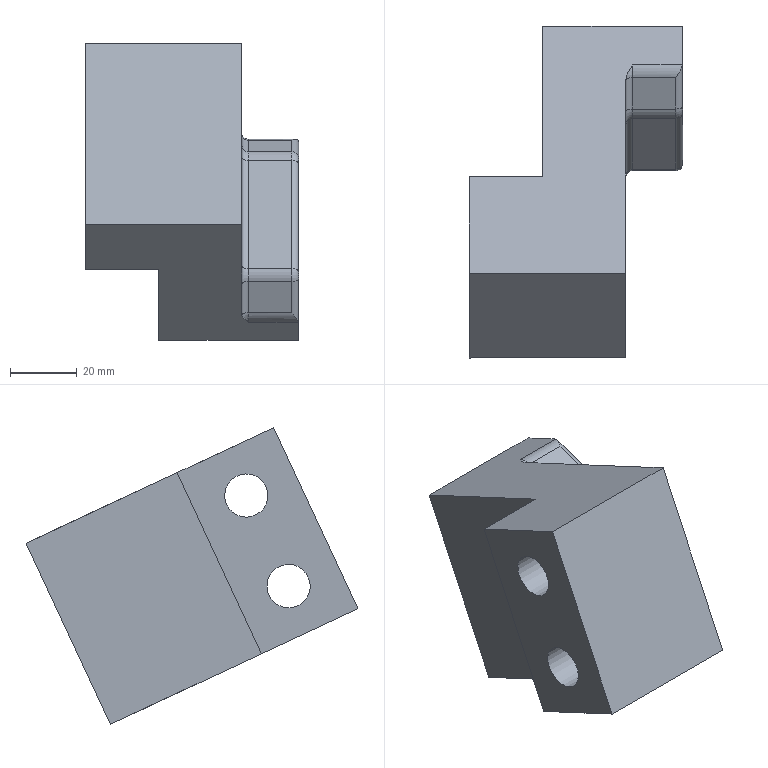Part | NX | features MAIN_BODY 2 | 1 solid | 34 faces | box 64 x 99.674 x 89.033 mm | volume 166732 mm3 | plane 14 | cylinder 14 | torus 6 | commonest cylinder face diameters 4 x6 10 x4 13 x2 20 x2
STEP:
#1=CARTESIAN_POINT('',(570.,631.034,-80.229));
#2=VERTEX_POINT('',#1);
#3=CARTESIAN_POINT('',(570.,656.391,-25.851));
#4=VERTEX_POINT('',#3);
#5=CARTESIAN_POINT('',(570.,631.034,-80.229));
#6=DIRECTION('',(0.,0.4226,0.9063));
#7=VECTOR('',#6,1000.);
#8=LINE('',#5,#7);
#9=EDGE_CURVE('',#2,#4,#8,.T.);
#10=ORIENTED_EDGE('',*,*,#9,.T.);
#11=CARTESIAN_POINT('',(570.,701.706,-46.982));
#12=VERTEX_POINT('',#11);
#13=CARTESIAN_POINT('',(570.,701.706,-46.982));
#14=DIRECTION('',(0.,-0.9063,0.4226));
#15=VECTOR('',#14,1000.);
#16=LINE('',#13,#15);
#17=EDGE_CURVE('',#12,#4,#16,.T.);
#18=ORIENTED_EDGE('',*,*,#17,.F.);
#19=CARTESIAN_POINT('',(570.,676.349,-101.36));
#20=VERTEX_POINT('',#19);
#21=CARTESIAN_POINT('',(570.,657.331,-142.144));
#22=DIRECTION('',(0.,0.4226,0.9063));
#23=VECTOR('',#22,1000.);
#24=LINE('',#21,#23);
#25=EDGE_CURVE('',#20,#12,#24,.T.);
#26=ORIENTED_EDGE('',*,*,#25,.F.);
#27=CARTESIAN_POINT('',(570.,676.349,-101.36));
#28=DIRECTION('',(0.,0.9063,-0.4226));
#29=VECTOR('',#28,1000.);
#30=LINE('',#27,#29);
#31=EDGE_CURVE('',#20,#2,#30,.F.);
#32=ORIENTED_EDGE('',*,*,#31,.T.);
#33=EDGE_LOOP('',(#10,#18,#26,#32));
#34=FACE_BOUND('',#33,.T.);
#35=CARTESIAN_POINT('',(570.,657.331,-142.144));
#36=DIRECTION('',(1.,0.,0.));
#37=DIRECTION('',(0.,-0.8192,-0.5736));
#38=AXIS2_PLACEMENT_3D('',#35,#36,#37);
#39=PLANE('',#38);
#40=ADVANCED_FACE('',(#34),#39,.F.);
#41=CARTESIAN_POINT('',(597.,689.989,-41.518));
#42=VERTEX_POINT('',#41);
#43=CARTESIAN_POINT('',(611.927,689.989,-41.518));
#44=VERTEX_POINT('',#43);
#45=CARTESIAN_POINT('',(563.,689.989,-41.518));
#46=DIRECTION('',(1.,0.,0.));
#47=VECTOR('',#46,1000.);
#48=LINE('',#45,#47);
#49=EDGE_CURVE('',#42,#44,#48,.T.);
#50=ORIENTED_EDGE('',*,*,#49,.T.);
#51=CARTESIAN_POINT('',(612.,690.675,-41.838));
#52=VERTEX_POINT('',#51);
#53=CARTESIAN_POINT('',(610.,690.675,-41.838));
#54=DIRECTION('',(0.,0.4226,0.9063));
#55=DIRECTION('',(0.,-0.9063,0.4226));
#56=AXIS2_PLACEMENT_3D('',#53,#54,#55);
#57=ELLIPSE('',#56,2.828,2.);
#58=EDGE_CURVE('',#44,#52,#57,.T.);
#59=ORIENTED_EDGE('',*,*,#58,.T.);
#60=CARTESIAN_POINT('',(612.,701.706,-46.982));
#61=VERTEX_POINT('',#60);
#62=CARTESIAN_POINT('',(612.,701.706,-46.982));
#63=DIRECTION('',(0.,-0.9063,0.4226));
#64=VECTOR('',#63,1000.);
#65=LINE('',#62,#64);
#66=EDGE_CURVE('',#61,#52,#65,.T.);
#67=ORIENTED_EDGE('',*,*,#66,.F.);
#68=CARTESIAN_POINT('',(563.,701.706,-46.982));
#69=DIRECTION('',(1.,0.,0.));
#70=VECTOR('',#69,1000.);
#71=LINE('',#68,#70);
#72=EDGE_CURVE('',#12,#61,#71,.T.);
#73=ORIENTED_EDGE('',*,*,#72,.F.);
#74=ORIENTED_EDGE('',*,*,#17,.T.);
#75=CARTESIAN_POINT('',(548.,656.391,-25.851));
#76=VERTEX_POINT('',#75);
#77=CARTESIAN_POINT('',(570.,656.391,-25.851));
#78=DIRECTION('',(1.,0.,0.));
#79=VECTOR('',#78,1000.);
#80=LINE('',#77,#79);
#81=EDGE_CURVE('',#4,#76,#80,.F.);
#82=ORIENTED_EDGE('',*,*,#81,.T.);
#83=CARTESIAN_POINT('',(548.,627.389,-12.327));
#84=VERTEX_POINT('',#83);
#85=CARTESIAN_POINT('',(548.,627.389,-12.327));
#86=DIRECTION('',(0.,0.9063,-0.4226));
#87=VECTOR('',#86,1000.);
#88=LINE('',#85,#87);
#89=EDGE_CURVE('',#84,#76,#88,.T.);
#90=ORIENTED_EDGE('',*,*,#89,.F.);
#91=CARTESIAN_POINT('',(595.,627.389,-12.327));
#92=VERTEX_POINT('',#91);
#93=CARTESIAN_POINT('',(563.,627.389,-12.327));
#94=DIRECTION('',(-1.,0.,0.));
#95=VECTOR('',#94,1000.);
#96=LINE('',#93,#95);
#97=EDGE_CURVE('',#84,#92,#96,.F.);
#98=ORIENTED_EDGE('',*,*,#97,.T.);
#99=CARTESIAN_POINT('',(595.,685.549,-39.447));
#100=VERTEX_POINT('',#99);
#101=CARTESIAN_POINT('',(595.,679.049,-36.416));
#102=DIRECTION('',(0.,-0.9063,0.4226));
#103=VECTOR('',#102,1000.);
#104=LINE('',#101,#103);
#105=EDGE_CURVE('',#100,#92,#104,.T.);
#106=ORIENTED_EDGE('',*,*,#105,.F.);
#107=CARTESIAN_POINT('',(595.,685.549,-39.447));
#108=CARTESIAN_POINT('',(595.,686.371,-39.831));
#109=CARTESIAN_POINT('',(595.571,687.945,-40.564));
#110=CARTESIAN_POINT('',(596.522,689.304,-41.198));
#111=CARTESIAN_POINT('',(597.,689.989,-41.518));
#112=B_SPLINE_CURVE_WITH_KNOTS('',3,(#107,#108,#109,#110,#111),.UNSPECIFIED.,.F.,.F.,(4,1,4),(0.,0.002683,0.005365),.UNSPECIFIED.);
#113=EDGE_CURVE('',#100,#42,#112,.T.);
#114=ORIENTED_EDGE('',*,*,#113,.T.);
#115=EDGE_LOOP('',(#50,#59,#67,#73,#74,#82,#90,#98,#106,#114));
#116=FACE_BOUND('',#115,.T.);
#117=CARTESIAN_POINT('',(563.,701.706,-46.982));
#118=DIRECTION('',(0.,0.4226,0.9063));
#119=DIRECTION('',(0.,-0.9063,0.4226));
#120=AXIS2_PLACEMENT_3D('',#117,#118,#119);
#121=PLANE('',#120);
#122=ADVANCED_FACE('',(#116),#121,.T.);
#123=CARTESIAN_POINT('',(548.,602.032,-66.705));
#124=VERTEX_POINT('',#123);
#125=CARTESIAN_POINT('',(595.,602.032,-66.705));
#126=VERTEX_POINT('',#125);
#127=CARTESIAN_POINT('',(563.,602.032,-66.705));
#128=DIRECTION('',(1.,0.,0.));
#129=VECTOR('',#128,1000.);
#130=LINE('',#127,#129);
#131=EDGE_CURVE('',#124,#126,#130,.T.);
#132=ORIENTED_EDGE('',*,*,#131,.T.);
#133=CARTESIAN_POINT('',(595.,583.014,-107.489));
#134=DIRECTION('',(0.,-0.4226,-0.9063));
#135=VECTOR('',#134,1000.);
#136=LINE('',#133,#135);
#137=EDGE_CURVE('',#126,#92,#136,.F.);
#138=ORIENTED_EDGE('',*,*,#137,.T.);
#139=ORIENTED_EDGE('',*,*,#97,.F.);
#140=CARTESIAN_POINT('',(548.,602.032,-66.705));
#141=DIRECTION('',(0.,0.4226,0.9063));
#142=VECTOR('',#141,1000.);
#143=LINE('',#140,#142);
#144=EDGE_CURVE('',#124,#84,#143,.T.);
#145=ORIENTED_EDGE('',*,*,#144,.F.);
#146=EDGE_LOOP('',(#132,#138,#139,#145));
#147=FACE_BOUND('',#146,.T.);
#148=CARTESIAN_POINT('',(563.,583.014,-107.489));
#149=DIRECTION('',(0.,0.9063,-0.4226));
#150=DIRECTION('',(0.,0.4226,0.9063));
#151=AXIS2_PLACEMENT_3D('',#148,#149,#150);
#152=PLANE('',#151);
#153=ADVANCED_FACE('',(#147),#152,.F.);
#154=CARTESIAN_POINT('',(612.,676.349,-101.36));
#155=VERTEX_POINT('',#154);
#156=CARTESIAN_POINT('',(612.,665.318,-96.216));
#157=VERTEX_POINT('',#156);
#158=CARTESIAN_POINT('',(612.,676.349,-101.36));
#159=DIRECTION('',(0.,0.9063,-0.4226));
#160=VECTOR('',#159,1000.);
#161=LINE('',#158,#160);
#162=EDGE_CURVE('',#155,#157,#161,.F.);
#163=ORIENTED_EDGE('',*,*,#162,.T.);
#164=CARTESIAN_POINT('',(611.927,664.632,-95.896));
#165=VERTEX_POINT('',#164);
#166=CARTESIAN_POINT('',(610.,665.318,-96.216));
#167=DIRECTION('',(0.,0.4226,0.9063));
#168=DIRECTION('',(0.,-0.9063,0.4226));
#169=AXIS2_PLACEMENT_3D('',#166,#167,#168);
#170=ELLIPSE('',#169,2.828,2.);
#171=EDGE_CURVE('',#157,#165,#170,.F.);
#172=ORIENTED_EDGE('',*,*,#171,.T.);
#173=CARTESIAN_POINT('',(597.,664.632,-95.896));
#174=VERTEX_POINT('',#173);
#175=CARTESIAN_POINT('',(563.,664.632,-95.896));
#176=DIRECTION('',(1.,0.,0.));
#177=VECTOR('',#176,1000.);
#178=LINE('',#175,#177);
#179=EDGE_CURVE('',#165,#174,#178,.F.);
#180=ORIENTED_EDGE('',*,*,#179,.T.);
#181=CARTESIAN_POINT('',(595.,660.192,-93.826));
#182=VERTEX_POINT('',#181);
#183=CARTESIAN_POINT('',(595.,660.192,-93.826));
#184=CARTESIAN_POINT('',(595.,661.014,-94.209));
#185=CARTESIAN_POINT('',(595.571,662.587,-94.943));
#186=CARTESIAN_POINT('',(596.522,663.947,-95.577));
#187=CARTESIAN_POINT('',(597.,664.632,-95.896));
#188=B_SPLINE_CURVE_WITH_KNOTS('',3,(#183,#184,#185,#186,#187),.UNSPECIFIED.,.F.,.F.,(4,1,4),(0.,0.002683,0.005365),.UNSPECIFIED.);
#189=EDGE_CURVE('',#174,#182,#188,.F.);
#190=ORIENTED_EDGE('',*,*,#189,.T.);
#191=CARTESIAN_POINT('',(595.,653.692,-90.795));
#192=DIRECTION('',(0.,-0.9063,0.4226));
#193=VECTOR('',#192,1000.);
#194=LINE('',#191,#193);
#195=EDGE_CURVE('',#182,#126,#194,.T.);
#196=ORIENTED_EDGE('',*,*,#195,.T.);
#197=ORIENTED_EDGE('',*,*,#131,.F.);
#198=CARTESIAN_POINT('',(548.,631.034,-80.229));
#199=VERTEX_POINT('',#198);
#200=CARTESIAN_POINT('',(548.,602.032,-66.705));
#201=DIRECTION('',(0.,0.9063,-0.4226));
#202=VECTOR('',#201,1000.);
#203=LINE('',#200,#202);
#204=EDGE_CURVE('',#124,#199,#203,.T.);
#205=ORIENTED_EDGE('',*,*,#204,.T.);
#206=CARTESIAN_POINT('',(570.,631.034,-80.229));
#207=DIRECTION('',(1.,0.,0.));
#208=VECTOR('',#207,1000.);
#209=LINE('',#206,#208);
#210=EDGE_CURVE('',#2,#199,#209,.F.);
#211=ORIENTED_EDGE('',*,*,#210,.F.);
#212=ORIENTED_EDGE('',*,*,#31,.F.);
#213=CARTESIAN_POINT('',(563.,676.349,-101.36));
#214=DIRECTION('',(-1.,0.,0.));
#215=VECTOR('',#214,1000.);
#216=LINE('',#213,#215);
#217=EDGE_CURVE('',#20,#155,#216,.F.);
#218=ORIENTED_EDGE('',*,*,#217,.T.);
#219=EDGE_LOOP('',(#163,#172,#180,#190,#196,#197,#205,#211,#212,#218));
#220=FACE_BOUND('',#219,.T.);
#221=CARTESIAN_POINT('',(563.,676.349,-101.36));
#222=DIRECTION('',(0.,0.4226,0.9063));
#223=DIRECTION('',(0.,-0.9063,0.4226));
#224=AXIS2_PLACEMENT_3D('',#221,#222,#223);
#225=PLANE('',#224);
#226=ADVANCED_FACE('',(#220),#225,.F.);
#227=CARTESIAN_POINT('',(612.,660.606,-80.7));
#228=VERTEX_POINT('',#227);
#229=CARTESIAN_POINT('',(612.,660.506,-82.994));
#230=VERTEX_POINT('',#229);
#231=CARTESIAN_POINT('',(612.,663.325,-81.968));
#232=DIRECTION('',(1.,0.,0.));
#233=DIRECTION('',(0.,-0.8192,-0.5736));
#234=AXIS2_PLACEMENT_3D('',#231,#232,#233);
#235=CIRCLE('',#234,3.);
#236=EDGE_CURVE('',#228,#230,#235,.T.);
#237=ORIENTED_EDGE('',*,*,#236,.T.);
#238=CARTESIAN_POINT('',(612.,679.145,-134.205));
#239=DIRECTION('',(0.,-0.342,0.9397));
#240=VECTOR('',#239,1000.);
#241=LINE('',#238,#240);
#242=EDGE_CURVE('',#230,#157,#241,.F.);
#243=ORIENTED_EDGE('',*,*,#242,.T.);
#244=ORIENTED_EDGE('',*,*,#162,.F.);
#245=CARTESIAN_POINT('',(612.,657.331,-142.144));
#246=DIRECTION('',(0.,0.4226,0.9063));
#247=VECTOR('',#246,1000.);
#248=LINE('',#245,#247);
#249=EDGE_CURVE('',#155,#61,#248,.T.);
#250=ORIENTED_EDGE('',*,*,#249,.T.);
#251=ORIENTED_EDGE('',*,*,#66,.T.);
#252=CARTESIAN_POINT('',(612.,677.453,-46.65));
#253=VERTEX_POINT('',#252);
#254=CARTESIAN_POINT('',(612.,628.994,-64.288));
#255=DIRECTION('',(0.,-0.9397,-0.342));
#256=VECTOR('',#255,1000.);
#257=LINE('',#254,#256);
#258=EDGE_CURVE('',#52,#253,#257,.T.);
#259=ORIENTED_EDGE('',*,*,#258,.T.);
#260=CARTESIAN_POINT('',(612.,675.76,-48.202));
#261=VERTEX_POINT('',#260);
#262=CARTESIAN_POINT('',(612.,678.479,-49.469));
#263=DIRECTION('',(1.,0.,0.));
#264=DIRECTION('',(0.,-0.8192,-0.5736));
#265=AXIS2_PLACEMENT_3D('',#262,#263,#264);
#266=CIRCLE('',#265,3.);
#267=EDGE_CURVE('',#253,#261,#266,.T.);
#268=ORIENTED_EDGE('',*,*,#267,.T.);
#269=CARTESIAN_POINT('',(612.,636.486,-132.424));
#270=DIRECTION('',(0.,0.4226,0.9063));
#271=VECTOR('',#270,1000.);
#272=LINE('',#269,#271);
#273=EDGE_CURVE('',#261,#228,#272,.F.);
#274=ORIENTED_EDGE('',*,*,#273,.T.);
#275=EDGE_LOOP('',(#237,#243,#244,#250,#251,#259,#268,#274));
#276=FACE_BOUND('',#275,.T.);
#277=CARTESIAN_POINT('',(612.,657.331,-142.144));
#278=DIRECTION('',(1.,0.,0.));
#279=DIRECTION('',(0.,-0.8192,-0.5736));
#280=AXIS2_PLACEMENT_3D('',#277,#278,#279);
#281=PLANE('',#280);
#282=ADVANCED_FACE('',(#276),#281,.T.);
#283=ORIENTED_EDGE('',*,*,#217,.F.);
#284=ORIENTED_EDGE('',*,*,#25,.T.);
#285=ORIENTED_EDGE('',*,*,#72,.T.);
#286=ORIENTED_EDGE('',*,*,#249,.F.);
#287=EDGE_LOOP('',(#283,#284,#285,#286));
#288=FACE_BOUND('',#287,.T.);
#289=CARTESIAN_POINT('',(563.,657.331,-142.144));
#290=DIRECTION('',(0.,0.9063,-0.4226));
#291=DIRECTION('',(0.,0.4226,0.9063));
#292=AXIS2_PLACEMENT_3D('',#289,#290,#291);
#293=PLANE('',#292);
#294=ADVANCED_FACE('',(#288),#293,.T.);
#295=CARTESIAN_POINT('',(597.,658.793,-79.855));
#296=VERTEX_POINT('',#295);
#297=CARTESIAN_POINT('',(610.,658.793,-79.855));
#298=VERTEX_POINT('',#297);
#299=CARTESIAN_POINT('',(563.,658.793,-79.855));
#300=DIRECTION('',(-1.,0.,0.));
#301=VECTOR('',#300,1000.);
#302=LINE('',#299,#301);
#303=EDGE_CURVE('',#296,#298,#302,.F.);
#304=ORIENTED_EDGE('',*,*,#303,.T.);
#305=CARTESIAN_POINT('',(610.,673.947,-47.356));
#306=VERTEX_POINT('',#305);
#307=CARTESIAN_POINT('',(610.,653.692,-90.795));
#308=DIRECTION('',(0.,-0.4226,-0.9063));
#309=VECTOR('',#308,1000.);
#310=LINE('',#307,#309);
#311=EDGE_CURVE('',#298,#306,#310,.F.);
#312=ORIENTED_EDGE('',*,*,#311,.T.);
#313=CARTESIAN_POINT('',(597.,673.947,-47.356));
#314=VERTEX_POINT('',#313);
#315=CARTESIAN_POINT('',(563.,673.947,-47.356));
#316=DIRECTION('',(-1.,0.,0.));
#317=VECTOR('',#316,1000.);
#318=LINE('',#315,#317);
#319=EDGE_CURVE('',#306,#314,#318,.T.);
#320=ORIENTED_EDGE('',*,*,#319,.T.);
#321=CARTESIAN_POINT('',(597.,658.793,-79.855));
#322=DIRECTION('',(0.,0.4226,0.9063));
#323=VECTOR('',#322,1000.);
#324=LINE('',#321,#323);
#325=EDGE_CURVE('',#314,#296,#324,.F.);
#326=ORIENTED_EDGE('',*,*,#325,.T.);
#327=EDGE_LOOP('',(#304,#312,#320,#326));
#328=FACE_BOUND('',#327,.T.);
#329=CARTESIAN_POINT('',(563.,653.692,-90.795));
#330=DIRECTION('',(0.,0.9063,-0.4226));
#331=DIRECTION('',(0.,0.4226,0.9063));
#332=AXIS2_PLACEMENT_3D('',#329,#330,#331);
#333=PLANE('',#332);
#334=ADVANCED_FACE('',(#328),#333,.F.);
#335=CARTESIAN_POINT('',(595.,625.46,-50.213));
#336=VERTEX_POINT('',#335);
#337=CARTESIAN_POINT('',(595.,622.872,-59.873));
#338=DIRECTION('',(-1.,0.,0.));
#339=DIRECTION('',(0.,0.2588,0.9659));
#340=AXIS2_PLACEMENT_3D('',#337,#338,#339);
#341=CIRCLE('',#340,10.);
#342=EDGE_CURVE('',#336,#336,#341,.T.);
#343=ORIENTED_EDGE('',*,*,#342,.T.);
#344=EDGE_LOOP('',(#343));
#345=FACE_BOUND('',#344,.T.);
#346=CARTESIAN_POINT('',(595.,638.139,-23.024));
#347=VERTEX_POINT('',#346);
#348=CARTESIAN_POINT('',(595.,635.551,-32.683));
#349=DIRECTION('',(-1.,0.,0.));
#350=DIRECTION('',(0.,0.2588,0.9659));
#351=AXIS2_PLACEMENT_3D('',#348,#349,#350);
#352=CIRCLE('',#351,10.);
#353=EDGE_CURVE('',#347,#347,#352,.T.);
#354=ORIENTED_EDGE('',*,*,#353,.T.);
#355=EDGE_LOOP('',(#354));
#356=FACE_BOUND('',#355,.T.);
#357=ORIENTED_EDGE('',*,*,#195,.F.);
#358=CARTESIAN_POINT('',(595.,660.167,-93.759));
#359=VERTEX_POINT('',#358);
#360=CARTESIAN_POINT('',(595.,666.745,-91.365));
#361=DIRECTION('',(1.,0.,0.));
#362=DIRECTION('',(0.,-0.8192,-0.5736));
#363=AXIS2_PLACEMENT_3D('',#360,#361,#362);
#364=CIRCLE('',#363,7.);
#365=EDGE_CURVE('',#182,#359,#364,.F.);
#366=ORIENTED_EDGE('',*,*,#365,.T.);
#367=CARTESIAN_POINT('',(595.,656.747,-84.362));
#368=VERTEX_POINT('',#367);
#369=CARTESIAN_POINT('',(595.,656.747,-84.362));
#370=DIRECTION('',(0.,0.342,-0.9397));
#371=VECTOR('',#370,1000.);
#372=LINE('',#369,#371);
#373=EDGE_CURVE('',#359,#368,#372,.F.);
#374=ORIENTED_EDGE('',*,*,#373,.T.);
#375=CARTESIAN_POINT('',(595.,656.98,-79.009));
#376=VERTEX_POINT('',#375);
#377=CARTESIAN_POINT('',(595.,663.325,-81.968));
#378=DIRECTION('',(1.,0.,0.));
#379=DIRECTION('',(0.,-0.8192,-0.5736));
#380=AXIS2_PLACEMENT_3D('',#377,#378,#379);
#381=CIRCLE('',#380,7.);
#382=EDGE_CURVE('',#368,#376,#381,.F.);
#383=ORIENTED_EDGE('',*,*,#382,.T.);
#384=CARTESIAN_POINT('',(595.,672.135,-46.511));
#385=VERTEX_POINT('',#384);
#386=CARTESIAN_POINT('',(595.,672.135,-46.511));
#387=DIRECTION('',(0.,-0.4226,-0.9063));
#388=VECTOR('',#387,1000.);
#389=LINE('',#386,#388);
#390=EDGE_CURVE('',#376,#385,#389,.F.);
#391=ORIENTED_EDGE('',*,*,#390,.T.);
#392=CARTESIAN_POINT('',(595.,676.085,-42.892));
#393=VERTEX_POINT('',#392);
#394=CARTESIAN_POINT('',(595.,678.479,-49.469));
#395=DIRECTION('',(1.,0.,0.));
#396=DIRECTION('',(0.,-0.8192,-0.5736));
#397=AXIS2_PLACEMENT_3D('',#394,#395,#396);
#398=CIRCLE('',#397,7.);
#399=EDGE_CURVE('',#385,#393,#398,.F.);
#400=ORIENTED_EDGE('',*,*,#399,.T.);
#401=CARTESIAN_POINT('',(595.,685.482,-39.471));
#402=VERTEX_POINT('',#401);
#403=CARTESIAN_POINT('',(595.,685.482,-39.471));
#404=DIRECTION('',(0.,0.9397,0.342));
#405=VECTOR('',#404,1000.);
#406=LINE('',#403,#405);
#407=EDGE_CURVE('',#393,#402,#406,.T.);
#408=ORIENTED_EDGE('',*,*,#407,.T.);
#409=CARTESIAN_POINT('',(595.,687.876,-46.049));
#410=DIRECTION('',(1.,0.,0.));
#411=DIRECTION('',(0.,-0.8192,-0.5736));
#412=AXIS2_PLACEMENT_3D('',#409,#410,#411);
#413=CIRCLE('',#412,7.);
#414=EDGE_CURVE('',#402,#100,#413,.F.);
#415=ORIENTED_EDGE('',*,*,#414,.T.);
#416=ORIENTED_EDGE('',*,*,#105,.T.);
#417=ORIENTED_EDGE('',*,*,#137,.F.);
#418=EDGE_LOOP('',(#357,#366,#374,#383,#391,#400,#408,#415,#416,#417));
#419=FACE_BOUND('',#418,.T.);
#420=CARTESIAN_POINT('',(595.,653.692,-90.795));
#421=DIRECTION('',(1.,0.,0.));
#422=DIRECTION('',(0.,-0.8192,-0.5736));
#423=AXIS2_PLACEMENT_3D('',#420,#421,#422);
#424=PLANE('',#423);
#425=ADVANCED_FACE('',(#345,#356,#419),#424,.T.);
#426=CARTESIAN_POINT('',(597.,662.046,-93.075));
#427=VERTEX_POINT('',#426);
#428=CARTESIAN_POINT('',(610.,662.046,-93.075));
#429=VERTEX_POINT('',#428);
#430=CARTESIAN_POINT('',(563.,662.046,-93.075));
#431=DIRECTION('',(1.,0.,0.));
#432=VECTOR('',#431,1000.);
#433=LINE('',#430,#432);
#434=EDGE_CURVE('',#427,#429,#433,.T.);
#435=ORIENTED_EDGE('',*,*,#434,.T.);
#436=CARTESIAN_POINT('',(610.,658.626,-83.678));
#437=VERTEX_POINT('',#436);
#438=CARTESIAN_POINT('',(610.,662.755,-95.021));
#439=DIRECTION('',(0.,0.342,-0.9397));
#440=VECTOR('',#439,1000.);
#441=LINE('',#438,#440);
#442=EDGE_CURVE('',#429,#437,#441,.F.);
#443=ORIENTED_EDGE('',*,*,#442,.T.);
#444=CARTESIAN_POINT('',(597.,658.626,-83.678));
#445=VERTEX_POINT('',#444);
#446=CARTESIAN_POINT('',(563.,658.626,-83.678));
#447=DIRECTION('',(-1.,0.,0.));
#448=VECTOR('',#447,1000.);
#449=LINE('',#446,#448);
#450=EDGE_CURVE('',#437,#445,#449,.T.);
#451=ORIENTED_EDGE('',*,*,#450,.T.);
#452=CARTESIAN_POINT('',(597.,662.046,-93.075));
#453=DIRECTION('',(0.,-0.342,0.9397));
#454=VECTOR('',#453,1000.);
#455=LINE('',#452,#454);
#456=EDGE_CURVE('',#445,#427,#455,.F.);
#457=ORIENTED_EDGE('',*,*,#456,.T.);
#458=EDGE_LOOP('',(#435,#443,#451,#457));
#459=FACE_BOUND('',#458,.T.);
#460=CARTESIAN_POINT('',(563.,662.755,-95.021));
#461=DIRECTION('',(0.,0.9397,0.342));
#462=DIRECTION('',(0.,-0.342,0.9397));
#463=AXIS2_PLACEMENT_3D('',#460,#461,#462);
#464=PLANE('',#463);
#465=ADVANCED_FACE('',(#459),#464,.F.);
#466=CARTESIAN_POINT('',(597.,676.769,-44.771));
#467=VERTEX_POINT('',#466);
#468=CARTESIAN_POINT('',(610.,676.769,-44.771));
#469=VERTEX_POINT('',#468);
#470=CARTESIAN_POINT('',(563.,676.769,-44.771));
#471=DIRECTION('',(1.,0.,0.));
#472=VECTOR('',#471,1000.);
#473=LINE('',#470,#472);
#474=EDGE_CURVE('',#467,#469,#473,.T.);
#475=ORIENTED_EDGE('',*,*,#474,.T.);
#476=CARTESIAN_POINT('',(610.,686.166,-41.351));
#477=VERTEX_POINT('',#476);
#478=CARTESIAN_POINT('',(610.,674.823,-45.479));
#479=DIRECTION('',(0.,-0.9397,-0.342));
#480=VECTOR('',#479,1000.);
#481=LINE('',#478,#480);
#482=EDGE_CURVE('',#469,#477,#481,.F.);
#483=ORIENTED_EDGE('',*,*,#482,.T.);
#484=CARTESIAN_POINT('',(597.,686.166,-41.351));
#485=VERTEX_POINT('',#484);
#486=CARTESIAN_POINT('',(563.,686.166,-41.351));
#487=DIRECTION('',(1.,0.,0.));
#488=VECTOR('',#487,1000.);
#489=LINE('',#486,#488);
#490=EDGE_CURVE('',#477,#485,#489,.F.);
#491=ORIENTED_EDGE('',*,*,#490,.T.);
#492=CARTESIAN_POINT('',(597.,676.769,-44.771));
#493=DIRECTION('',(0.,0.9397,0.342));
#494=VECTOR('',#493,1000.);
#495=LINE('',#492,#494);
#496=EDGE_CURVE('',#485,#467,#495,.F.);
#497=ORIENTED_EDGE('',*,*,#496,.T.);
#498=EDGE_LOOP('',(#475,#483,#491,#497));
#499=FACE_BOUND('',#498,.T.);
#500=CARTESIAN_POINT('',(563.,674.823,-45.479));
#501=DIRECTION('',(0.,-0.342,0.9397));
#502=DIRECTION('',(0.,-0.9397,-0.342));
#503=AXIS2_PLACEMENT_3D('',#500,#501,#502);
#504=PLANE('',#503);
#505=ADVANCED_FACE('',(#499),#504,.T.);
#506=ORIENTED_EDGE('',*,*,#490,.F.);
#507=CARTESIAN_POINT('',(611.927,689.989,-41.518));
#508=CARTESIAN_POINT('',(611.641,688.67,-40.903));
#509=CARTESIAN_POINT('',(610.781,687.326,-40.928));
#510=CARTESIAN_POINT('',(610.,686.166,-41.351));
#511=B_SPLINE_CURVE_WITH_KNOTS('',3,(#507,#508,#509,#510),.UNSPECIFIED.,.F.,.F.,(4,4),(0.,0.004383),.UNSPECIFIED.);
#512=EDGE_CURVE('',#477,#44,#511,.F.);
#513=ORIENTED_EDGE('',*,*,#512,.T.);
#514=ORIENTED_EDGE('',*,*,#49,.F.);
#515=CARTESIAN_POINT('',(597.,687.876,-46.049));
#516=DIRECTION('',(1.,0.,0.));
#517=DIRECTION('',(0.,-0.8192,-0.5736));
#518=AXIS2_PLACEMENT_3D('',#515,#516,#517);
#519=CIRCLE('',#518,5.);
#520=EDGE_CURVE('',#42,#485,#519,.T.);
#521=ORIENTED_EDGE('',*,*,#520,.T.);
#522=EDGE_LOOP('',(#506,#513,#514,#521));
#523=FACE_BOUND('',#522,.T.);
#524=CARTESIAN_POINT('',(563.,687.876,-46.049));
#525=DIRECTION('',(1.,0.,0.));
#526=DIRECTION('',(0.,-0.8192,-0.5736));
#527=AXIS2_PLACEMENT_3D('',#524,#525,#526);
#528=CYLINDRICAL_SURFACE('',#527,5.);
#529=ADVANCED_FACE('',(#523),#528,.T.);
#530=ORIENTED_EDGE('',*,*,#319,.F.);
#531=CARTESIAN_POINT('',(610.,678.479,-49.469));
#532=DIRECTION('',(1.,0.,0.));
#533=DIRECTION('',(0.,-0.8192,-0.5736));
#534=AXIS2_PLACEMENT_3D('',#531,#532,#533);
#535=CIRCLE('',#534,5.);
#536=EDGE_CURVE('',#306,#469,#535,.F.);
#537=ORIENTED_EDGE('',*,*,#536,.T.);
#538=ORIENTED_EDGE('',*,*,#474,.F.);
#539=CARTESIAN_POINT('',(597.,678.479,-49.469));
#540=DIRECTION('',(1.,0.,0.));
#541=DIRECTION('',(0.,-0.8192,-0.5736));
#542=AXIS2_PLACEMENT_3D('',#539,#540,#541);
#543=CIRCLE('',#542,5.);
#544=EDGE_CURVE('',#467,#314,#543,.T.);
#545=ORIENTED_EDGE('',*,*,#544,.T.);
#546=EDGE_LOOP('',(#530,#537,#538,#545));
#547=FACE_BOUND('',#546,.T.);
#548=CARTESIAN_POINT('',(563.,678.479,-49.469));
#549=DIRECTION('',(1.,0.,0.));
#550=DIRECTION('',(0.,-0.8192,-0.5736));
#551=AXIS2_PLACEMENT_3D('',#548,#549,#550);
#552=CYLINDRICAL_SURFACE('',#551,5.);
#553=ADVANCED_FACE('',(#547),#552,.T.);
#554=ORIENTED_EDGE('',*,*,#450,.F.);
#555=CARTESIAN_POINT('',(610.,663.325,-81.968));
#556=DIRECTION('',(1.,0.,0.));
#557=DIRECTION('',(0.,-0.8192,-0.5736));
#558=AXIS2_PLACEMENT_3D('',#555,#556,#557);
#559=CIRCLE('',#558,5.);
#560=EDGE_CURVE('',#437,#298,#559,.F.);
#561=ORIENTED_EDGE('',*,*,#560,.T.);
#562=ORIENTED_EDGE('',*,*,#303,.F.);
#563=CARTESIAN_POINT('',(597.,663.325,-81.968));
#564=DIRECTION('',(1.,0.,0.));
#565=DIRECTION('',(0.,-0.8192,-0.5736));
#566=AXIS2_PLACEMENT_3D('',#563,#564,#565);
#567=CIRCLE('',#566,5.);
#568=EDGE_CURVE('',#296,#445,#567,.T.);
#569=ORIENTED_EDGE('',*,*,#568,.T.);
#570=EDGE_LOOP('',(#554,#561,#562,#569));
#571=FACE_BOUND('',#570,.T.);
#572=CARTESIAN_POINT('',(563.,663.325,-81.968));
#573=DIRECTION('',(1.,0.,0.));
#574=DIRECTION('',(0.,-0.8192,-0.5736));
#575=AXIS2_PLACEMENT_3D('',#572,#573,#574);
#576=CYLINDRICAL_SURFACE('',#575,5.);
#577=ADVANCED_FACE('',(#571),#576,.T.);
#578=ORIENTED_EDGE('',*,*,#179,.F.);
#579=CARTESIAN_POINT('',(611.927,664.632,-95.896));
#580=CARTESIAN_POINT('',(611.641,663.313,-95.281));
#581=CARTESIAN_POINT('',(610.781,662.469,-94.235));
#582=CARTESIAN_POINT('',(610.,662.046,-93.075));
#583=B_SPLINE_CURVE_WITH_KNOTS('',3,(#579,#580,#581,#582),.UNSPECIFIED.,.F.,.F.,(4,4),(0.,0.004383),.UNSPECIFIED.);
#584=EDGE_CURVE('',#165,#429,#583,.T.);
#585=ORIENTED_EDGE('',*,*,#584,.T.);
#586=ORIENTED_EDGE('',*,*,#434,.F.);
#587=CARTESIAN_POINT('',(597.,666.745,-91.365));
#588=DIRECTION('',(1.,0.,0.));
#589=DIRECTION('',(0.,-0.8192,-0.5736));
#590=AXIS2_PLACEMENT_3D('',#587,#588,#589);
#591=CIRCLE('',#590,5.);
#592=EDGE_CURVE('',#427,#174,#591,.T.);
#593=ORIENTED_EDGE('',*,*,#592,.T.);
#594=EDGE_LOOP('',(#578,#585,#586,#593));
#595=FACE_BOUND('',#594,.T.);
#596=CARTESIAN_POINT('',(563.,666.745,-91.365));
#597=DIRECTION('',(-1.,0.,0.));
#598=DIRECTION('',(0.,0.8192,0.5736));
#599=AXIS2_PLACEMENT_3D('',#596,#597,#598);
#600=CYLINDRICAL_SURFACE('',#599,5.);
#601=ADVANCED_FACE('',(#595),#600,.T.);
#602=ORIENTED_EDGE('',*,*,#113,.F.);
#603=ORIENTED_EDGE('',*,*,#414,.F.);
#604=CARTESIAN_POINT('',(597.,685.482,-39.471));
#605=DIRECTION('',(0.,0.9397,0.342));
#606=DIRECTION('',(0.,-0.342,0.9397));
#607=AXIS2_PLACEMENT_3D('',#604,#605,#606);
#608=CIRCLE('',#607,2.);
#609=EDGE_CURVE('',#485,#402,#608,.T.);
#610=ORIENTED_EDGE('',*,*,#609,.F.);
#611=ORIENTED_EDGE('',*,*,#520,.F.);
#612=EDGE_LOOP('',(#602,#603,#610,#611));
#613=FACE_BOUND('',#612,.T.);
#614=CARTESIAN_POINT('',(597.,687.876,-46.049));
#615=DIRECTION('',(1.,0.,0.));
#616=DIRECTION('',(0.,-0.8192,-0.5736));
#617=AXIS2_PLACEMENT_3D('',#614,#615,#616);
#618=TOROIDAL_SURFACE('',#617,7.,2.);
#619=ADVANCED_FACE('',(#613),#618,.F.);
#620=ORIENTED_EDGE('',*,*,#609,.T.);
#621=ORIENTED_EDGE('',*,*,#407,.F.);
#622=CARTESIAN_POINT('',(597.,676.085,-42.892));
#623=DIRECTION('',(0.,0.9397,0.342));
#624=DIRECTION('',(0.,-0.342,0.9397));
#625=AXIS2_PLACEMENT_3D('',#622,#623,#624);
#626=CIRCLE('',#625,2.);
#627=EDGE_CURVE('',#467,#393,#626,.T.);
#628=ORIENTED_EDGE('',*,*,#627,.F.);
#629=ORIENTED_EDGE('',*,*,#496,.F.);
#630=EDGE_LOOP('',(#620,#621,#628,#629));
#631=FACE_BOUND('',#630,.T.);
#632=CARTESIAN_POINT('',(597.,640.915,-55.692));
#633=DIRECTION('',(0.,-0.9397,-0.342));
#634=DIRECTION('',(0.,0.342,-0.9397));
#635=AXIS2_PLACEMENT_3D('',#632,#633,#634);
#636=CYLINDRICAL_SURFACE('',#635,2.);
#637=ADVANCED_FACE('',(#631),#636,.F.);
#638=ORIENTED_EDGE('',*,*,#627,.T.);
#639=ORIENTED_EDGE('',*,*,#399,.F.);
#640=CARTESIAN_POINT('',(597.,672.135,-46.511));
#641=DIRECTION('',(0.,0.4226,0.9063));
#642=DIRECTION('',(0.,-0.9063,0.4226));
#643=AXIS2_PLACEMENT_3D('',#640,#641,#642);
#644=CIRCLE('',#643,2.);
#645=EDGE_CURVE('',#314,#385,#644,.T.);
#646=ORIENTED_EDGE('',*,*,#645,.F.);
#647=ORIENTED_EDGE('',*,*,#544,.F.);
#648=EDGE_LOOP('',(#638,#639,#646,#647));
#649=FACE_BOUND('',#648,.T.);
#650=CARTESIAN_POINT('',(597.,678.479,-49.469));
#651=DIRECTION('',(1.,0.,0.));
#652=DIRECTION('',(0.,-0.8192,-0.5736));
#653=AXIS2_PLACEMENT_3D('',#650,#651,#652);
#654=TOROIDAL_SURFACE('',#653,7.,2.);
#655=ADVANCED_FACE('',(#649),#654,.F.);
#656=ORIENTED_EDGE('',*,*,#645,.T.);
#657=ORIENTED_EDGE('',*,*,#390,.F.);
#658=CARTESIAN_POINT('',(597.,656.98,-79.009));
#659=DIRECTION('',(0.,0.4226,0.9063));
#660=DIRECTION('',(0.,-0.9063,0.4226));
#661=AXIS2_PLACEMENT_3D('',#658,#659,#660);
#662=CIRCLE('',#661,2.);
#663=EDGE_CURVE('',#296,#376,#662,.T.);
#664=ORIENTED_EDGE('',*,*,#663,.F.);
#665=ORIENTED_EDGE('',*,*,#325,.F.);
#666=EDGE_LOOP('',(#656,#657,#664,#665));
#667=FACE_BOUND('',#666,.T.);
#668=CARTESIAN_POINT('',(597.,651.879,-89.949));
#669=DIRECTION('',(0.,0.4226,0.9063));
#670=DIRECTION('',(0.,-0.9063,0.4226));
#671=AXIS2_PLACEMENT_3D('',#668,#669,#670);
#672=CYLINDRICAL_SURFACE('',#671,2.);
#673=ADVANCED_FACE('',(#667),#672,.F.);
#674=ORIENTED_EDGE('',*,*,#663,.T.);
#675=ORIENTED_EDGE('',*,*,#382,.F.);
#676=CARTESIAN_POINT('',(597.,656.747,-84.362));
#677=DIRECTION('',(0.,-0.342,0.9397));
#678=DIRECTION('',(0.,-0.9397,-0.342));
#679=AXIS2_PLACEMENT_3D('',#676,#677,#678);
#680=CIRCLE('',#679,2.);
#681=EDGE_CURVE('',#445,#368,#680,.T.);
#682=ORIENTED_EDGE('',*,*,#681,.F.);
#683=ORIENTED_EDGE('',*,*,#568,.F.);
#684=EDGE_LOOP('',(#674,#675,#682,#683));
#685=FACE_BOUND('',#684,.T.);
#686=CARTESIAN_POINT('',(597.,663.325,-81.968));
#687=DIRECTION('',(1.,0.,0.));
#688=DIRECTION('',(0.,-0.8192,-0.5736));
#689=AXIS2_PLACEMENT_3D('',#686,#687,#688);
#690=TOROIDAL_SURFACE('',#689,7.,2.);
#691=ADVANCED_FACE('',(#685),#690,.F.);
#692=ORIENTED_EDGE('',*,*,#681,.T.);
#693=ORIENTED_EDGE('',*,*,#373,.F.);
#694=CARTESIAN_POINT('',(597.,660.167,-93.759));
#695=DIRECTION('',(0.,-0.342,0.9397));
#696=DIRECTION('',(0.,-0.9397,-0.342));
#697=AXIS2_PLACEMENT_3D('',#694,#695,#696);
#698=CIRCLE('',#697,2.);
#699=EDGE_CURVE('',#427,#359,#698,.T.);
#700=ORIENTED_EDGE('',*,*,#699,.F.);
#701=ORIENTED_EDGE('',*,*,#456,.F.);
#702=EDGE_LOOP('',(#692,#693,#700,#701));
#703=FACE_BOUND('',#702,.T.);
#704=CARTESIAN_POINT('',(597.,658.457,-89.06));
#705=DIRECTION('',(0.,-0.342,0.9397));
#706=DIRECTION('',(0.,-0.9397,-0.342));
#707=AXIS2_PLACEMENT_3D('',#704,#705,#706);
#708=CYLINDRICAL_SURFACE('',#707,2.);
#709=ADVANCED_FACE('',(#703),#708,.F.);
#710=ORIENTED_EDGE('',*,*,#189,.F.);
#711=ORIENTED_EDGE('',*,*,#592,.F.);
#712=ORIENTED_EDGE('',*,*,#699,.T.);
#713=ORIENTED_EDGE('',*,*,#365,.F.);
#714=EDGE_LOOP('',(#710,#711,#712,#713));
#715=FACE_BOUND('',#714,.T.);
#716=CARTESIAN_POINT('',(597.,666.745,-91.365));
#717=DIRECTION('',(1.,0.,0.));
#718=DIRECTION('',(0.,-0.8192,-0.5736));
#719=AXIS2_PLACEMENT_3D('',#716,#717,#718);
#720=TOROIDAL_SURFACE('',#719,7.,2.);
#721=ADVANCED_FACE('',(#715),#720,.F.);
#722=ORIENTED_EDGE('',*,*,#512,.F.);
#723=ORIENTED_EDGE('',*,*,#482,.F.);
#724=CARTESIAN_POINT('',(610.,677.453,-46.65));
#725=DIRECTION('',(0.,-0.9397,-0.342));
#726=DIRECTION('',(0.,0.342,-0.9397));
#727=AXIS2_PLACEMENT_3D('',#724,#725,#726);
#728=CIRCLE('',#727,2.);
#729=EDGE_CURVE('',#253,#469,#728,.T.);
#730=ORIENTED_EDGE('',*,*,#729,.F.);
#731=ORIENTED_EDGE('',*,*,#258,.F.);
#732=ORIENTED_EDGE('',*,*,#58,.F.);
#733=EDGE_LOOP('',(#722,#723,#730,#731,#732));
#734=FACE_BOUND('',#733,.T.);
#735=CARTESIAN_POINT('',(610.,628.994,-64.288));
#736=DIRECTION('',(0.,-0.9397,-0.342));
#737=DIRECTION('',(0.,0.342,-0.9397));
#738=AXIS2_PLACEMENT_3D('',#735,#736,#737);
#739=CYLINDRICAL_SURFACE('',#738,2.);
#740=ADVANCED_FACE('',(#734),#739,.T.);
#741=ORIENTED_EDGE('',*,*,#729,.T.);
#742=ORIENTED_EDGE('',*,*,#536,.F.);
#743=CARTESIAN_POINT('',(610.,675.76,-48.202));
#744=DIRECTION('',(0.,-0.4226,-0.9063));
#745=DIRECTION('',(0.,0.9063,-0.4226));
#746=AXIS2_PLACEMENT_3D('',#743,#744,#745);
#747=CIRCLE('',#746,2.);
#748=EDGE_CURVE('',#261,#306,#747,.T.);
#749=ORIENTED_EDGE('',*,*,#748,.F.);
#750=ORIENTED_EDGE('',*,*,#267,.F.);
#751=EDGE_LOOP('',(#741,#742,#749,#750));
#752=FACE_BOUND('',#751,.T.);
#753=CARTESIAN_POINT('',(610.,678.479,-49.469));
#754=DIRECTION('',(1.,0.,0.));
#755=DIRECTION('',(0.,-0.8192,-0.5736));
#756=AXIS2_PLACEMENT_3D('',#753,#754,#755);
#757=TOROIDAL_SURFACE('',#756,3.,2.);
#758=ADVANCED_FACE('',(#752),#757,.T.);
#759=ORIENTED_EDGE('',*,*,#748,.T.);
#760=ORIENTED_EDGE('',*,*,#311,.F.);
#761=CARTESIAN_POINT('',(610.,660.606,-80.7));
#762=DIRECTION('',(0.,-0.4226,-0.9063));
#763=DIRECTION('',(0.,0.9063,-0.4226));
#764=AXIS2_PLACEMENT_3D('',#761,#762,#763);
#765=CIRCLE('',#764,2.);
#766=EDGE_CURVE('',#228,#298,#765,.T.);
#767=ORIENTED_EDGE('',*,*,#766,.F.);
#768=ORIENTED_EDGE('',*,*,#273,.F.);
#769=EDGE_LOOP('',(#759,#760,#767,#768));
#770=FACE_BOUND('',#769,.T.);
#771=CARTESIAN_POINT('',(610.,636.486,-132.424));
#772=DIRECTION('',(0.,0.4226,0.9063));
#773=DIRECTION('',(0.,-0.9063,0.4226));
#774=AXIS2_PLACEMENT_3D('',#771,#772,#773);
#775=CYLINDRICAL_SURFACE('',#774,2.);
#776=ADVANCED_FACE('',(#770),#775,.T.);
#777=ORIENTED_EDGE('',*,*,#171,.F.);
#778=ORIENTED_EDGE('',*,*,#242,.F.);
#779=CARTESIAN_POINT('',(610.,660.506,-82.994));
#780=DIRECTION('',(0.,-0.342,0.9397));
#781=DIRECTION('',(0.,-0.9397,-0.342));
#782=AXIS2_PLACEMENT_3D('',#779,#780,#781);
#783=CIRCLE('',#782,2.);
#784=EDGE_CURVE('',#437,#230,#783,.T.);
#785=ORIENTED_EDGE('',*,*,#784,.F.);
#786=ORIENTED_EDGE('',*,*,#442,.F.);
#787=ORIENTED_EDGE('',*,*,#584,.F.);
#788=EDGE_LOOP('',(#777,#778,#785,#786,#787));
#789=FACE_BOUND('',#788,.T.);
#790=CARTESIAN_POINT('',(610.,679.145,-134.205));
#791=DIRECTION('',(0.,-0.342,0.9397));
#792=DIRECTION('',(0.,-0.9397,-0.342));
#793=AXIS2_PLACEMENT_3D('',#790,#791,#792);
#794=CYLINDRICAL_SURFACE('',#793,2.);
#795=ADVANCED_FACE('',(#789),#794,.T.);
#796=ORIENTED_EDGE('',*,*,#766,.T.);
#797=ORIENTED_EDGE('',*,*,#560,.F.);
#798=ORIENTED_EDGE('',*,*,#784,.T.);
#799=ORIENTED_EDGE('',*,*,#236,.F.);
#800=EDGE_LOOP('',(#796,#797,#798,#799));
#801=FACE_BOUND('',#800,.T.);
#802=CARTESIAN_POINT('',(610.,663.325,-81.968));
#803=DIRECTION('',(1.,0.,0.));
#804=DIRECTION('',(0.,-0.8192,-0.5736));
#805=AXIS2_PLACEMENT_3D('',#802,#803,#804);
#806=TOROIDAL_SURFACE('',#805,3.,2.);
#807=ADVANCED_FACE('',(#801),#806,.T.);
#808=ORIENTED_EDGE('',*,*,#210,.T.);
#809=CARTESIAN_POINT('',(548.,631.034,-80.229));
#810=DIRECTION('',(0.,0.4226,0.9063));
#811=VECTOR('',#810,1000.);
#812=LINE('',#809,#811);
#813=EDGE_CURVE('',#199,#76,#812,.T.);
#814=ORIENTED_EDGE('',*,*,#813,.T.);
#815=ORIENTED_EDGE('',*,*,#81,.F.);
#816=ORIENTED_EDGE('',*,*,#9,.F.);
#817=EDGE_LOOP('',(#808,#814,#815,#816));
#818=FACE_BOUND('',#817,.T.);
#819=CARTESIAN_POINT('',(570.,631.034,-80.229));
#820=DIRECTION('',(0.,-0.9063,0.4226));
#821=DIRECTION('',(0.,0.4226,0.9063));
#822=AXIS2_PLACEMENT_3D('',#819,#820,#821);
#823=PLANE('',#822);
#824=ADVANCED_FACE('',(#818),#823,.F.);
#825=CARTESIAN_POINT('',(548.,624.555,-53.594));
#826=VERTEX_POINT('',#825);
#827=CARTESIAN_POINT('',(548.,622.872,-59.873));
#828=DIRECTION('',(-1.,0.,0.));
#829=DIRECTION('',(0.,0.2588,0.9659));
#830=AXIS2_PLACEMENT_3D('',#827,#828,#829);
#831=CIRCLE('',#830,6.5);
#832=EDGE_CURVE('',#826,#826,#831,.T.);
#833=ORIENTED_EDGE('',*,*,#832,.F.);
#834=EDGE_LOOP('',(#833));
#835=FACE_BOUND('',#834,.T.);
#836=CARTESIAN_POINT('',(548.,637.233,-26.405));
#837=VERTEX_POINT('',#836);
#838=CARTESIAN_POINT('',(548.,635.551,-32.683));
#839=DIRECTION('',(-1.,0.,0.));
#840=DIRECTION('',(0.,0.2588,0.9659));
#841=AXIS2_PLACEMENT_3D('',#838,#839,#840);
#842=CIRCLE('',#841,6.5);
#843=EDGE_CURVE('',#837,#837,#842,.T.);
#844=ORIENTED_EDGE('',*,*,#843,.F.);
#845=EDGE_LOOP('',(#844));
#846=FACE_BOUND('',#845,.T.);
#847=ORIENTED_EDGE('',*,*,#813,.F.);
#848=ORIENTED_EDGE('',*,*,#204,.F.);
#849=ORIENTED_EDGE('',*,*,#144,.T.);
#850=ORIENTED_EDGE('',*,*,#89,.T.);
#851=EDGE_LOOP('',(#847,#848,#849,#850));
#852=FACE_BOUND('',#851,.T.);
#853=CARTESIAN_POINT('',(548.,602.032,-66.705));
#854=DIRECTION('',(-1.,0.,0.));
#855=DIRECTION('',(0.,0.2588,0.9659));
#856=AXIS2_PLACEMENT_3D('',#853,#854,#855);
#857=PLANE('',#856);
#858=ADVANCED_FACE('',(#835,#846,#852),#857,.T.);
#859=ORIENTED_EDGE('',*,*,#843,.T.);
#860=EDGE_LOOP('',(#859));
#861=FACE_BOUND('',#860,.T.);
#862=CARTESIAN_POINT('',(568.,637.233,-26.405));
#863=VERTEX_POINT('',#862);
#864=CARTESIAN_POINT('',(568.,635.551,-32.683));
#865=DIRECTION('',(-1.,0.,0.));
#866=DIRECTION('',(0.,0.2588,0.9659));
#867=AXIS2_PLACEMENT_3D('',#864,#865,#866);
#868=CIRCLE('',#867,6.5);
#869=EDGE_CURVE('',#863,#863,#868,.T.);
#870=ORIENTED_EDGE('',*,*,#869,.F.);
#871=EDGE_LOOP('',(#870));
#872=FACE_BOUND('',#871,.T.);
#873=CARTESIAN_POINT('',(495.,635.551,-32.683));
#874=DIRECTION('',(-1.,0.,0.));
#875=DIRECTION('',(0.,0.2588,0.9659));
#876=AXIS2_PLACEMENT_3D('',#873,#874,#875);
#877=CYLINDRICAL_SURFACE('',#876,6.5);
#878=ADVANCED_FACE('',(#861,#872),#877,.F.);
#879=ORIENTED_EDGE('',*,*,#869,.T.);
#880=EDGE_LOOP('',(#879));
#881=FACE_BOUND('',#880,.T.);
#882=CARTESIAN_POINT('',(568.,638.139,-23.024));
#883=VERTEX_POINT('',#882);
#884=CARTESIAN_POINT('',(568.,635.551,-32.683));
#885=DIRECTION('',(-1.,0.,0.));
#886=DIRECTION('',(0.,0.2588,0.9659));
#887=AXIS2_PLACEMENT_3D('',#884,#885,#886);
#888=CIRCLE('',#887,10.);
#889=EDGE_CURVE('',#883,#883,#888,.T.);
#890=ORIENTED_EDGE('',*,*,#889,.F.);
#891=EDGE_LOOP('',(#890));
#892=FACE_BOUND('',#891,.T.);
#893=CARTESIAN_POINT('',(568.,635.551,-32.683));
#894=DIRECTION('',(-1.,0.,0.));
#895=DIRECTION('',(0.,0.2588,0.9659));
#896=AXIS2_PLACEMENT_3D('',#893,#894,#895);
#897=PLANE('',#896);
#898=ADVANCED_FACE('',(#881,#892),#897,.F.);
#899=ORIENTED_EDGE('',*,*,#889,.T.);
#900=EDGE_LOOP('',(#899));
#901=FACE_BOUND('',#900,.T.);
#902=ORIENTED_EDGE('',*,*,#353,.F.);
#903=EDGE_LOOP('',(#902));
#904=FACE_BOUND('',#903,.T.);
#905=CARTESIAN_POINT('',(595.,635.551,-32.683));
#906=DIRECTION('',(-1.,0.,0.));
#907=DIRECTION('',(0.,0.2588,0.9659));
#908=AXIS2_PLACEMENT_3D('',#905,#906,#907);
#909=CYLINDRICAL_SURFACE('',#908,10.);
#910=ADVANCED_FACE('',(#901,#904),#909,.F.);
#911=ORIENTED_EDGE('',*,*,#832,.T.);
#912=EDGE_LOOP('',(#911));
#913=FACE_BOUND('',#912,.T.);
#914=CARTESIAN_POINT('',(568.,624.555,-53.594));
#915=VERTEX_POINT('',#914);
#916=CARTESIAN_POINT('',(568.,622.872,-59.873));
#917=DIRECTION('',(-1.,0.,0.));
#918=DIRECTION('',(0.,0.2588,0.9659));
#919=AXIS2_PLACEMENT_3D('',#916,#917,#918);
#920=CIRCLE('',#919,6.5);
#921=EDGE_CURVE('',#915,#915,#920,.T.);
#922=ORIENTED_EDGE('',*,*,#921,.F.);
#923=EDGE_LOOP('',(#922));
#924=FACE_BOUND('',#923,.T.);
#925=CARTESIAN_POINT('',(495.,622.872,-59.873));
#926=DIRECTION('',(-1.,0.,0.));
#927=DIRECTION('',(0.,0.2588,0.9659));
#928=AXIS2_PLACEMENT_3D('',#925,#926,#927);
#929=CYLINDRICAL_SURFACE('',#928,6.5);
#930=ADVANCED_FACE('',(#913,#924),#929,.F.);
#931=ORIENTED_EDGE('',*,*,#921,.T.);
#932=EDGE_LOOP('',(#931));
#933=FACE_BOUND('',#932,.T.);
#934=CARTESIAN_POINT('',(568.,625.46,-50.213));
#935=VERTEX_POINT('',#934);
#936=CARTESIAN_POINT('',(568.,622.872,-59.873));
#937=DIRECTION('',(-1.,0.,0.));
#938=DIRECTION('',(0.,0.2588,0.9659));
#939=AXIS2_PLACEMENT_3D('',#936,#937,#938);
#940=CIRCLE('',#939,10.);
#941=EDGE_CURVE('',#935,#935,#940,.T.);
#942=ORIENTED_EDGE('',*,*,#941,.F.);
#943=EDGE_LOOP('',(#942));
#944=FACE_BOUND('',#943,.T.);
#945=CARTESIAN_POINT('',(568.,622.872,-59.873));
#946=DIRECTION('',(-1.,0.,0.));
#947=DIRECTION('',(0.,0.2588,0.9659));
#948=AXIS2_PLACEMENT_3D('',#945,#946,#947);
#949=PLANE('',#948);
#950=ADVANCED_FACE('',(#933,#944),#949,.F.);
#951=ORIENTED_EDGE('',*,*,#941,.T.);
#952=EDGE_LOOP('',(#951));
#953=FACE_BOUND('',#952,.T.);
#954=ORIENTED_EDGE('',*,*,#342,.F.);
#955=EDGE_LOOP('',(#954));
#956=FACE_BOUND('',#955,.T.);
#957=CARTESIAN_POINT('',(595.,622.872,-59.873));
#958=DIRECTION('',(-1.,0.,0.));
#959=DIRECTION('',(0.,0.2588,0.9659));
#960=AXIS2_PLACEMENT_3D('',#957,#958,#959);
#961=CYLINDRICAL_SURFACE('',#960,10.);
#962=ADVANCED_FACE('',(#953,#956),#961,.F.);
#963=CLOSED_SHELL('',(#40,#122,#153,#226,#282,#294,#334,#425,#465,#505,#529,#553,#577,#601,#619,#637,#655,#673,#691,#709,#721,#740,#758,#776,#795,#807,#824,#858,#878,#898,#910,#930,#950,#962));
#964=MANIFOLD_SOLID_BREP('',#963);
#965=(LENGTH_UNIT()NAMED_UNIT(*)SI_UNIT(.MILLI.,.METRE.));
#966=UNCERTAINTY_MEASURE_WITH_UNIT(LENGTH_MEASURE(0.0508),#965,'','');
#967=(NAMED_UNIT(*)PLANE_ANGLE_UNIT()SI_UNIT($,.RADIAN.));
#968=(NAMED_UNIT(*)SI_UNIT($,.STERADIAN.)SOLID_ANGLE_UNIT());
#969=(GEOMETRIC_REPRESENTATION_CONTEXT(3)GLOBAL_UNCERTAINTY_ASSIGNED_CONTEXT((#966))GLOBAL_UNIT_ASSIGNED_CONTEXT((#965,#967,#968))REPRESENTATION_CONTEXT('',''));
#970=ADVANCED_BREP_SHAPE_REPRESENTATION('',(#964),#969);